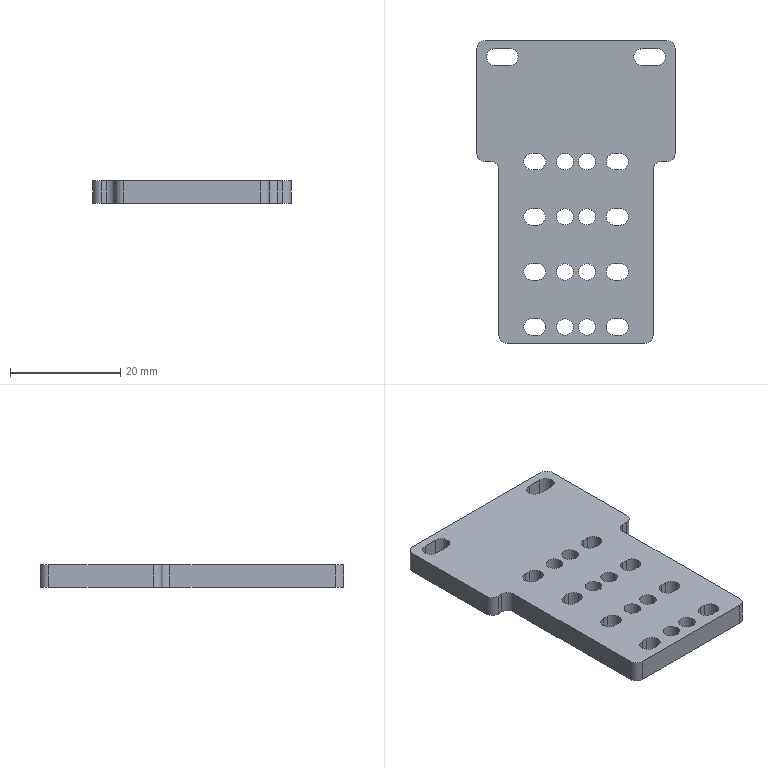Part | SolidWorks | features ICE 2, Extrusion 1, Fillet 1 | 1 solid | 84 faces | box 36 x 55 x 4 mm | volume 6185 mm3 | cylinder 54 | plane 30 | commonest cylinder face diameters 3 x54